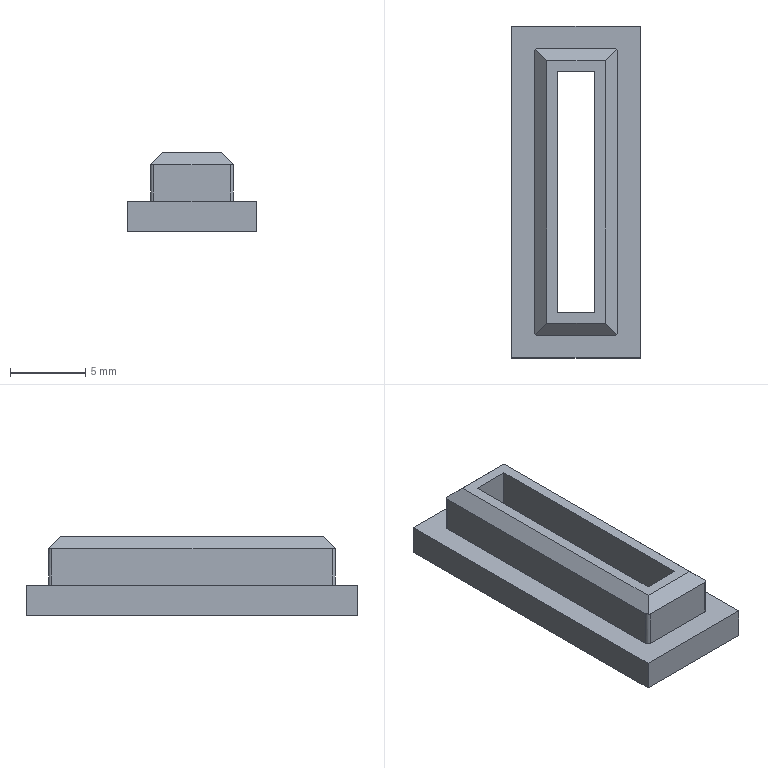Part | NX | features BREP 1 | 1 solid | 23 faces | box 8.5 x 22 x 5.2 mm | volume 485.324 mm3 | plane 19 | cylinder 4 | commonest cylinder face diameters 0.4 x4
STEP:
#1=CARTESIAN_POINT('',(-10.019,-6.965,4.4));
#2=VERTEX_POINT('',#1);
#3=CARTESIAN_POINT('',(-10.077,-7.106,4.459));
#4=VERTEX_POINT('',#3);
#5=CARTESIAN_POINT('',(-10.219,-6.965,4.6));
#6=DIRECTION('',(-0.7071,0.,-0.7071));
#7=DIRECTION('',(0.7071,0.,-0.7071));
#8=AXIS2_PLACEMENT_3D('',#5,#6,#7);
#9=ELLIPSE('',#8,0.2828,0.2);
#10=EDGE_CURVE('',#2,#4,#9,.T.);
#11=ORIENTED_EDGE('',*,*,#10,.F.);
#12=CARTESIAN_POINT('',(-10.019,11.635,4.4));
#13=VERTEX_POINT('',#12);
#14=CARTESIAN_POINT('',(-10.019,11.635,4.4));
#15=DIRECTION('',(0.,-1.,0.));
#16=VECTOR('',#15,1000.);
#17=LINE('',#14,#16);
#18=EDGE_CURVE('',#13,#2,#17,.T.);
#19=ORIENTED_EDGE('',*,*,#18,.F.);
#20=CARTESIAN_POINT('',(-10.078,11.777,4.459));
#21=VERTEX_POINT('',#20);
#22=CARTESIAN_POINT('',(-10.219,11.635,4.6));
#23=DIRECTION('',(-0.7071,0.,-0.7071));
#24=DIRECTION('',(0.7071,0.,-0.7071));
#25=AXIS2_PLACEMENT_3D('',#22,#23,#24);
#26=ELLIPSE('',#25,0.2828,0.2);
#27=EDGE_CURVE('',#21,#13,#26,.T.);
#28=ORIENTED_EDGE('',*,*,#27,.F.);
#29=CARTESIAN_POINT('',(-10.819,11.034,5.2));
#30=VERTEX_POINT('',#29);
#31=CARTESIAN_POINT('',(-10.819,11.034,5.2));
#32=DIRECTION('',(0.5767,0.5786,-0.5767));
#33=VECTOR('',#32,1000.);
#34=LINE('',#31,#33);
#35=EDGE_CURVE('',#30,#21,#34,.T.);
#36=ORIENTED_EDGE('',*,*,#35,.F.);
#37=CARTESIAN_POINT('',(-10.819,-6.367,5.2));
#38=VERTEX_POINT('',#37);
#39=CARTESIAN_POINT('',(-10.819,-6.367,5.2));
#40=DIRECTION('',(0.,1.,0.));
#41=VECTOR('',#40,1000.);
#42=LINE('',#39,#41);
#43=EDGE_CURVE('',#38,#30,#42,.T.);
#44=ORIENTED_EDGE('',*,*,#43,.F.);
#45=CARTESIAN_POINT('',(-10.077,-7.106,4.459));
#46=DIRECTION('',(-0.578,0.5761,0.578));
#47=VECTOR('',#46,1000.);
#48=LINE('',#45,#47);
#49=EDGE_CURVE('',#4,#38,#48,.T.);
#50=ORIENTED_EDGE('',*,*,#49,.F.);
#51=EDGE_LOOP('',(#11,#19,#28,#36,#44,#50));
#52=FACE_BOUND('',#51,.T.);
#53=CARTESIAN_POINT('',(-10.077,-8.665,4.459));
#54=DIRECTION('',(-0.7071,0.,-0.7071));
#55=DIRECTION('',(-0.7071,0.,0.7071));
#56=AXIS2_PLACEMENT_3D('',#53,#54,#55);
#57=PLANE('',#56);
#58=ADVANCED_FACE('',(#52),#57,.F.);
#59=CARTESIAN_POINT('',(-15.519,11.635,4.4));
#60=VERTEX_POINT('',#59);
#61=CARTESIAN_POINT('',(-15.46,11.777,4.459));
#62=VERTEX_POINT('',#61);
#63=CARTESIAN_POINT('',(-15.319,11.635,4.6));
#64=DIRECTION('',(0.7071,0.,-0.7071));
#65=DIRECTION('',(-0.7071,0.,-0.7071));
#66=AXIS2_PLACEMENT_3D('',#63,#64,#65);
#67=ELLIPSE('',#66,0.2828,0.2);
#68=EDGE_CURVE('',#60,#62,#67,.T.);
#69=ORIENTED_EDGE('',*,*,#68,.F.);
#70=CARTESIAN_POINT('',(-15.519,-6.965,4.4));
#71=VERTEX_POINT('',#70);
#72=CARTESIAN_POINT('',(-15.519,-6.965,4.4));
#73=DIRECTION('',(0.,1.,0.));
#74=VECTOR('',#73,1000.);
#75=LINE('',#72,#74);
#76=EDGE_CURVE('',#71,#60,#75,.T.);
#77=ORIENTED_EDGE('',*,*,#76,.F.);
#78=CARTESIAN_POINT('',(-15.46,-7.106,4.459));
#79=VERTEX_POINT('',#78);
#80=CARTESIAN_POINT('',(-15.319,-6.965,4.6));
#81=DIRECTION('',(0.7071,0.,-0.7071));
#82=DIRECTION('',(-0.7071,0.,-0.7071));
#83=AXIS2_PLACEMENT_3D('',#80,#81,#82);
#84=ELLIPSE('',#83,0.2828,0.2);
#85=EDGE_CURVE('',#79,#71,#84,.T.);
#86=ORIENTED_EDGE('',*,*,#85,.F.);
#87=CARTESIAN_POINT('',(-14.719,-6.367,5.2));
#88=VERTEX_POINT('',#87);
#89=CARTESIAN_POINT('',(-14.719,-6.367,5.2));
#90=DIRECTION('',(-0.578,-0.5761,-0.578));
#91=VECTOR('',#90,1000.);
#92=LINE('',#89,#91);
#93=EDGE_CURVE('',#88,#79,#92,.T.);
#94=ORIENTED_EDGE('',*,*,#93,.F.);
#95=CARTESIAN_POINT('',(-14.719,11.034,5.2));
#96=VERTEX_POINT('',#95);
#97=CARTESIAN_POINT('',(-14.719,11.034,5.2));
#98=DIRECTION('',(0.,-1.,0.));
#99=VECTOR('',#98,1000.);
#100=LINE('',#97,#99);
#101=EDGE_CURVE('',#96,#88,#100,.T.);
#102=ORIENTED_EDGE('',*,*,#101,.F.);
#103=CARTESIAN_POINT('',(-15.46,11.777,4.459));
#104=DIRECTION('',(0.5767,-0.5786,0.5767));
#105=VECTOR('',#104,1000.);
#106=LINE('',#103,#105);
#107=EDGE_CURVE('',#62,#96,#106,.T.);
#108=ORIENTED_EDGE('',*,*,#107,.F.);
#109=EDGE_LOOP('',(#69,#77,#86,#94,#102,#108));
#110=FACE_BOUND('',#109,.T.);
#111=CARTESIAN_POINT('',(-15.46,-8.665,4.459));
#112=DIRECTION('',(0.7071,0.,-0.7071));
#113=DIRECTION('',(-0.7071,0.,-0.7071));
#114=AXIS2_PLACEMENT_3D('',#111,#112,#113);
#115=PLANE('',#114);
#116=ADVANCED_FACE('',(#110),#115,.F.);
#117=ORIENTED_EDGE('',*,*,#10,.T.);
#118=CARTESIAN_POINT('',(-10.219,-7.165,4.4));
#119=VERTEX_POINT('',#118);
#120=CARTESIAN_POINT('',(-10.219,-6.965,4.601));
#121=DIRECTION('',(0.,0.7083,-0.7059));
#122=DIRECTION('',(0.,-0.7059,-0.7083));
#123=AXIS2_PLACEMENT_3D('',#120,#121,#122);
#124=ELLIPSE('',#123,0.2833,0.2);
#125=EDGE_CURVE('',#4,#119,#124,.T.);
#126=ORIENTED_EDGE('',*,*,#125,.T.);
#127=CARTESIAN_POINT('',(-10.219,-7.165,2.));
#128=VERTEX_POINT('',#127);
#129=CARTESIAN_POINT('',(-10.219,-7.165,2.));
#130=DIRECTION('',(0.,0.,1.));
#131=VECTOR('',#130,1000.);
#132=LINE('',#129,#131);
#133=EDGE_CURVE('',#128,#119,#132,.T.);
#134=ORIENTED_EDGE('',*,*,#133,.F.);
#135=CARTESIAN_POINT('',(-10.019,-6.965,2.));
#136=VERTEX_POINT('',#135);
#137=CARTESIAN_POINT('',(-10.219,-6.965,2.));
#138=DIRECTION('',(0.,0.,-1.));
#139=DIRECTION('',(0.,-1.,0.));
#140=AXIS2_PLACEMENT_3D('',#137,#138,#139);
#141=CIRCLE('',#140,0.2);
#142=EDGE_CURVE('',#136,#128,#141,.T.);
#143=ORIENTED_EDGE('',*,*,#142,.F.);
#144=CARTESIAN_POINT('',(-10.019,-6.965,2.));
#145=DIRECTION('',(0.,0.,1.));
#146=VECTOR('',#145,1000.);
#147=LINE('',#144,#146);
#148=EDGE_CURVE('',#136,#2,#147,.T.);
#149=ORIENTED_EDGE('',*,*,#148,.T.);
#150=EDGE_LOOP('',(#117,#126,#134,#143,#149));
#151=FACE_BOUND('',#150,.T.);
#152=CARTESIAN_POINT('',(-10.219,-6.965,2.));
#153=DIRECTION('',(0.,0.,1.));
#154=DIRECTION('',(0.,-1.,0.));
#155=AXIS2_PLACEMENT_3D('',#152,#153,#154);
#156=CYLINDRICAL_SURFACE('',#155,0.2);
#157=ADVANCED_FACE('',(#151),#156,.T.);
#158=ORIENTED_EDGE('',*,*,#68,.T.);
#159=CARTESIAN_POINT('',(-15.319,11.835,4.401));
#160=VERTEX_POINT('',#159);
#161=CARTESIAN_POINT('',(-15.319,11.635,4.6));
#162=DIRECTION('',(0.,-0.7059,-0.7083));
#163=DIRECTION('',(0.,0.7083,-0.7059));
#164=AXIS2_PLACEMENT_3D('',#161,#162,#163);
#165=ELLIPSE('',#164,0.2824,0.2);
#166=EDGE_CURVE('',#62,#160,#165,.T.);
#167=ORIENTED_EDGE('',*,*,#166,.T.);
#168=CARTESIAN_POINT('',(-15.319,11.835,2.));
#169=VERTEX_POINT('',#168);
#170=CARTESIAN_POINT('',(-15.319,11.835,2.));
#171=DIRECTION('',(0.,0.,1.));
#172=VECTOR('',#171,1000.);
#173=LINE('',#170,#172);
#174=EDGE_CURVE('',#169,#160,#173,.T.);
#175=ORIENTED_EDGE('',*,*,#174,.F.);
#176=CARTESIAN_POINT('',(-15.519,11.635,2.));
#177=VERTEX_POINT('',#176);
#178=CARTESIAN_POINT('',(-15.319,11.635,2.));
#179=DIRECTION('',(0.,0.,-1.));
#180=DIRECTION('',(0.,1.,0.));
#181=AXIS2_PLACEMENT_3D('',#178,#179,#180);
#182=CIRCLE('',#181,0.2);
#183=EDGE_CURVE('',#177,#169,#182,.T.);
#184=ORIENTED_EDGE('',*,*,#183,.F.);
#185=CARTESIAN_POINT('',(-15.519,11.635,2.));
#186=DIRECTION('',(0.,0.,1.));
#187=VECTOR('',#186,1000.);
#188=LINE('',#185,#187);
#189=EDGE_CURVE('',#177,#60,#188,.T.);
#190=ORIENTED_EDGE('',*,*,#189,.T.);
#191=EDGE_LOOP('',(#158,#167,#175,#184,#190));
#192=FACE_BOUND('',#191,.T.);
#193=CARTESIAN_POINT('',(-15.319,11.635,2.));
#194=DIRECTION('',(0.,0.,1.));
#195=DIRECTION('',(0.,1.,0.));
#196=AXIS2_PLACEMENT_3D('',#193,#194,#195);
#197=CYLINDRICAL_SURFACE('',#196,0.2);
#198=ADVANCED_FACE('',(#192),#197,.T.);
#199=ORIENTED_EDGE('',*,*,#43,.T.);
#200=CARTESIAN_POINT('',(-10.819,11.034,5.2));
#201=DIRECTION('',(-1.,0.,0.));
#202=VECTOR('',#201,1000.);
#203=LINE('',#200,#202);
#204=EDGE_CURVE('',#30,#96,#203,.T.);
#205=ORIENTED_EDGE('',*,*,#204,.T.);
#206=ORIENTED_EDGE('',*,*,#101,.T.);
#207=CARTESIAN_POINT('',(-14.719,-6.367,5.2));
#208=DIRECTION('',(1.,0.,0.));
#209=VECTOR('',#208,1000.);
#210=LINE('',#207,#209);
#211=EDGE_CURVE('',#88,#38,#210,.T.);
#212=ORIENTED_EDGE('',*,*,#211,.T.);
#213=EDGE_LOOP('',(#199,#205,#206,#212));
#214=FACE_BOUND('',#213,.T.);
#215=CARTESIAN_POINT('',(-14.019,-5.665,5.2));
#216=VERTEX_POINT('',#215);
#217=CARTESIAN_POINT('',(-14.019,10.335,5.2));
#218=VERTEX_POINT('',#217);
#219=CARTESIAN_POINT('',(-14.019,-5.665,5.2));
#220=DIRECTION('',(0.,1.,0.));
#221=VECTOR('',#220,1000.);
#222=LINE('',#219,#221);
#223=EDGE_CURVE('',#216,#218,#222,.T.);
#224=ORIENTED_EDGE('',*,*,#223,.T.);
#225=CARTESIAN_POINT('',(-11.519,10.335,5.2));
#226=VERTEX_POINT('',#225);
#227=CARTESIAN_POINT('',(-14.019,10.335,5.2));
#228=DIRECTION('',(1.,0.,0.));
#229=VECTOR('',#228,1000.);
#230=LINE('',#227,#229);
#231=EDGE_CURVE('',#218,#226,#230,.T.);
#232=ORIENTED_EDGE('',*,*,#231,.T.);
#233=CARTESIAN_POINT('',(-11.519,-5.665,5.2));
#234=VERTEX_POINT('',#233);
#235=CARTESIAN_POINT('',(-11.519,10.335,5.2));
#236=DIRECTION('',(0.,-1.,0.));
#237=VECTOR('',#236,1000.);
#238=LINE('',#235,#237);
#239=EDGE_CURVE('',#226,#234,#238,.T.);
#240=ORIENTED_EDGE('',*,*,#239,.T.);
#241=CARTESIAN_POINT('',(-11.519,-5.665,5.2));
#242=DIRECTION('',(-1.,0.,0.));
#243=VECTOR('',#242,1000.);
#244=LINE('',#241,#243);
#245=EDGE_CURVE('',#234,#216,#244,.T.);
#246=ORIENTED_EDGE('',*,*,#245,.T.);
#247=EDGE_LOOP('',(#224,#232,#240,#246));
#248=FACE_BOUND('',#247,.T.);
#249=CARTESIAN_POINT('',(-12.769,-6.812,5.2));
#250=DIRECTION('',(0.,0.,1.));
#251=DIRECTION('',(1.,0.,0.));
#252=AXIS2_PLACEMENT_3D('',#249,#250,#251);
#253=PLANE('',#252);
#254=ADVANCED_FACE('',(#214,#248),#253,.T.);
#255=ORIENTED_EDGE('',*,*,#49,.T.);
#256=ORIENTED_EDGE('',*,*,#211,.F.);
#257=ORIENTED_EDGE('',*,*,#93,.T.);
#258=CARTESIAN_POINT('',(-15.319,-7.165,4.4));
#259=VERTEX_POINT('',#258);
#260=CARTESIAN_POINT('',(-15.319,-6.965,4.601));
#261=DIRECTION('',(0.,0.7083,-0.7059));
#262=DIRECTION('',(0.,-0.7059,-0.7083));
#263=AXIS2_PLACEMENT_3D('',#260,#261,#262);
#264=ELLIPSE('',#263,0.2833,0.2);
#265=EDGE_CURVE('',#259,#79,#264,.T.);
#266=ORIENTED_EDGE('',*,*,#265,.F.);
#267=CARTESIAN_POINT('',(-10.219,-7.165,4.4));
#268=DIRECTION('',(-1.,0.,0.));
#269=VECTOR('',#268,1000.);
#270=LINE('',#267,#269);
#271=EDGE_CURVE('',#119,#259,#270,.T.);
#272=ORIENTED_EDGE('',*,*,#271,.F.);
#273=ORIENTED_EDGE('',*,*,#125,.F.);
#274=EDGE_LOOP('',(#255,#256,#257,#266,#272,#273));
#275=FACE_BOUND('',#274,.T.);
#276=CARTESIAN_POINT('',(-10.019,-7.165,4.4));
#277=DIRECTION('',(0.,0.7083,-0.7059));
#278=DIRECTION('',(-1.,0.,0.));
#279=AXIS2_PLACEMENT_3D('',#276,#277,#278);
#280=PLANE('',#279);
#281=ADVANCED_FACE('',(#275),#280,.F.);
#282=ORIENTED_EDGE('',*,*,#85,.T.);
#283=CARTESIAN_POINT('',(-15.519,-6.965,2.));
#284=VERTEX_POINT('',#283);
#285=CARTESIAN_POINT('',(-15.519,-6.965,2.));
#286=DIRECTION('',(0.,0.,1.));
#287=VECTOR('',#286,1000.);
#288=LINE('',#285,#287);
#289=EDGE_CURVE('',#284,#71,#288,.T.);
#290=ORIENTED_EDGE('',*,*,#289,.F.);
#291=CARTESIAN_POINT('',(-15.319,-7.165,2.));
#292=VERTEX_POINT('',#291);
#293=CARTESIAN_POINT('',(-15.319,-6.965,2.));
#294=DIRECTION('',(0.,0.,-1.));
#295=DIRECTION('',(-1.,-0.000000001,0.));
#296=AXIS2_PLACEMENT_3D('',#293,#294,#295);
#297=CIRCLE('',#296,0.2);
#298=EDGE_CURVE('',#292,#284,#297,.T.);
#299=ORIENTED_EDGE('',*,*,#298,.F.);
#300=CARTESIAN_POINT('',(-15.319,-7.165,2.));
#301=DIRECTION('',(0.,0.,1.));
#302=VECTOR('',#301,1000.);
#303=LINE('',#300,#302);
#304=EDGE_CURVE('',#292,#259,#303,.T.);
#305=ORIENTED_EDGE('',*,*,#304,.T.);
#306=ORIENTED_EDGE('',*,*,#265,.T.);
#307=EDGE_LOOP('',(#282,#290,#299,#305,#306));
#308=FACE_BOUND('',#307,.T.);
#309=CARTESIAN_POINT('',(-15.319,-6.965,2.));
#310=DIRECTION('',(0.,0.,1.));
#311=DIRECTION('',(-1.,-0.000000001,0.));
#312=AXIS2_PLACEMENT_3D('',#309,#310,#311);
#313=CYLINDRICAL_SURFACE('',#312,0.2);
#314=ADVANCED_FACE('',(#308),#313,.T.);
#315=ORIENTED_EDGE('',*,*,#76,.T.);
#316=ORIENTED_EDGE('',*,*,#189,.F.);
#317=CARTESIAN_POINT('',(-15.519,-6.965,2.));
#318=DIRECTION('',(0.,1.,0.));
#319=VECTOR('',#318,1000.);
#320=LINE('',#317,#319);
#321=EDGE_CURVE('',#284,#177,#320,.T.);
#322=ORIENTED_EDGE('',*,*,#321,.F.);
#323=ORIENTED_EDGE('',*,*,#289,.T.);
#324=EDGE_LOOP('',(#315,#316,#322,#323));
#325=FACE_BOUND('',#324,.T.);
#326=CARTESIAN_POINT('',(-15.519,-6.965,2.));
#327=DIRECTION('',(-1.,0.,0.));
#328=DIRECTION('',(0.,0.,1.));
#329=AXIS2_PLACEMENT_3D('',#326,#327,#328);
#330=PLANE('',#329);
#331=ADVANCED_FACE('',(#325),#330,.T.);
#332=ORIENTED_EDGE('',*,*,#35,.T.);
#333=CARTESIAN_POINT('',(-10.219,11.835,4.401));
#334=VERTEX_POINT('',#333);
#335=CARTESIAN_POINT('',(-10.219,11.635,4.6));
#336=DIRECTION('',(0.,-0.7059,-0.7083));
#337=DIRECTION('',(0.,0.7083,-0.7059));
#338=AXIS2_PLACEMENT_3D('',#335,#336,#337);
#339=ELLIPSE('',#338,0.2824,0.2);
#340=EDGE_CURVE('',#334,#21,#339,.T.);
#341=ORIENTED_EDGE('',*,*,#340,.F.);
#342=CARTESIAN_POINT('',(-15.319,11.835,4.401));
#343=DIRECTION('',(1.,0.,0.));
#344=VECTOR('',#343,1000.);
#345=LINE('',#342,#344);
#346=EDGE_CURVE('',#160,#334,#345,.T.);
#347=ORIENTED_EDGE('',*,*,#346,.F.);
#348=ORIENTED_EDGE('',*,*,#166,.F.);
#349=ORIENTED_EDGE('',*,*,#107,.T.);
#350=ORIENTED_EDGE('',*,*,#204,.F.);
#351=EDGE_LOOP('',(#332,#341,#347,#348,#349,#350));
#352=FACE_BOUND('',#351,.T.);
#353=CARTESIAN_POINT('',(-10.019,11.034,5.2));
#354=DIRECTION('',(0.,-0.7059,-0.7083));
#355=DIRECTION('',(-1.,0.,0.));
#356=AXIS2_PLACEMENT_3D('',#353,#354,#355);
#357=PLANE('',#356);
#358=ADVANCED_FACE('',(#352),#357,.F.);
#359=ORIENTED_EDGE('',*,*,#27,.T.);
#360=CARTESIAN_POINT('',(-10.019,11.635,2.));
#361=VERTEX_POINT('',#360);
#362=CARTESIAN_POINT('',(-10.019,11.635,2.));
#363=DIRECTION('',(0.,0.,1.));
#364=VECTOR('',#363,1000.);
#365=LINE('',#362,#364);
#366=EDGE_CURVE('',#361,#13,#365,.T.);
#367=ORIENTED_EDGE('',*,*,#366,.F.);
#368=CARTESIAN_POINT('',(-10.219,11.835,2.));
#369=VERTEX_POINT('',#368);
#370=CARTESIAN_POINT('',(-10.219,11.635,2.));
#371=DIRECTION('',(0.,0.,-1.));
#372=DIRECTION('',(1.,0.,0.));
#373=AXIS2_PLACEMENT_3D('',#370,#371,#372);
#374=CIRCLE('',#373,0.2);
#375=EDGE_CURVE('',#369,#361,#374,.T.);
#376=ORIENTED_EDGE('',*,*,#375,.F.);
#377=CARTESIAN_POINT('',(-10.219,11.835,2.));
#378=DIRECTION('',(0.,0.,1.));
#379=VECTOR('',#378,1000.);
#380=LINE('',#377,#379);
#381=EDGE_CURVE('',#369,#334,#380,.T.);
#382=ORIENTED_EDGE('',*,*,#381,.T.);
#383=ORIENTED_EDGE('',*,*,#340,.T.);
#384=EDGE_LOOP('',(#359,#367,#376,#382,#383));
#385=FACE_BOUND('',#384,.T.);
#386=CARTESIAN_POINT('',(-10.219,11.635,2.));
#387=DIRECTION('',(0.,0.,1.));
#388=DIRECTION('',(1.,0.,0.));
#389=AXIS2_PLACEMENT_3D('',#386,#387,#388);
#390=CYLINDRICAL_SURFACE('',#389,0.2);
#391=ADVANCED_FACE('',(#385),#390,.T.);
#392=ORIENTED_EDGE('',*,*,#18,.T.);
#393=ORIENTED_EDGE('',*,*,#148,.F.);
#394=CARTESIAN_POINT('',(-10.019,11.635,2.));
#395=DIRECTION('',(0.,-1.,0.));
#396=VECTOR('',#395,1000.);
#397=LINE('',#394,#396);
#398=EDGE_CURVE('',#361,#136,#397,.T.);
#399=ORIENTED_EDGE('',*,*,#398,.F.);
#400=ORIENTED_EDGE('',*,*,#366,.T.);
#401=EDGE_LOOP('',(#392,#393,#399,#400));
#402=FACE_BOUND('',#401,.T.);
#403=CARTESIAN_POINT('',(-10.019,11.635,2.));
#404=DIRECTION('',(1.,0.,0.));
#405=DIRECTION('',(0.,0.,-1.));
#406=AXIS2_PLACEMENT_3D('',#403,#404,#405);
#407=PLANE('',#406);
#408=ADVANCED_FACE('',(#402),#407,.T.);
#409=ORIENTED_EDGE('',*,*,#223,.F.);
#410=CARTESIAN_POINT('',(-14.019,-5.665,0.));
#411=VERTEX_POINT('',#410);
#412=CARTESIAN_POINT('',(-14.019,-5.665,5.2));
#413=DIRECTION('',(0.,0.,-1.));
#414=VECTOR('',#413,1000.);
#415=LINE('',#412,#414);
#416=EDGE_CURVE('',#216,#411,#415,.T.);
#417=ORIENTED_EDGE('',*,*,#416,.T.);
#418=CARTESIAN_POINT('',(-14.019,10.335,0.));
#419=VERTEX_POINT('',#418);
#420=CARTESIAN_POINT('',(-14.019,10.335,0.));
#421=DIRECTION('',(0.,-1.,0.));
#422=VECTOR('',#421,1000.);
#423=LINE('',#420,#422);
#424=EDGE_CURVE('',#419,#411,#423,.T.);
#425=ORIENTED_EDGE('',*,*,#424,.F.);
#426=CARTESIAN_POINT('',(-14.019,10.335,0.));
#427=DIRECTION('',(0.,0.,1.));
#428=VECTOR('',#427,1000.);
#429=LINE('',#426,#428);
#430=EDGE_CURVE('',#419,#218,#429,.T.);
#431=ORIENTED_EDGE('',*,*,#430,.T.);
#432=EDGE_LOOP('',(#409,#417,#425,#431));
#433=FACE_BOUND('',#432,.T.);
#434=CARTESIAN_POINT('',(-14.019,-5.665,2.));
#435=DIRECTION('',(-1.,0.,0.));
#436=DIRECTION('',(0.,0.,1.));
#437=AXIS2_PLACEMENT_3D('',#434,#435,#436);
#438=PLANE('',#437);
#439=ADVANCED_FACE('',(#433),#438,.F.);
#440=ORIENTED_EDGE('',*,*,#231,.F.);
#441=ORIENTED_EDGE('',*,*,#430,.F.);
#442=CARTESIAN_POINT('',(-11.519,10.335,0.));
#443=VERTEX_POINT('',#442);
#444=CARTESIAN_POINT('',(-11.519,10.335,0.));
#445=DIRECTION('',(-1.,0.,0.));
#446=VECTOR('',#445,1000.);
#447=LINE('',#444,#446);
#448=EDGE_CURVE('',#443,#419,#447,.T.);
#449=ORIENTED_EDGE('',*,*,#448,.F.);
#450=CARTESIAN_POINT('',(-11.519,10.335,0.));
#451=DIRECTION('',(0.,0.,1.));
#452=VECTOR('',#451,1000.);
#453=LINE('',#450,#452);
#454=EDGE_CURVE('',#443,#226,#453,.T.);
#455=ORIENTED_EDGE('',*,*,#454,.T.);
#456=EDGE_LOOP('',(#440,#441,#449,#455));
#457=FACE_BOUND('',#456,.T.);
#458=CARTESIAN_POINT('',(-14.019,10.335,2.));
#459=DIRECTION('',(0.,1.,0.));
#460=DIRECTION('',(0.,0.,1.));
#461=AXIS2_PLACEMENT_3D('',#458,#459,#460);
#462=PLANE('',#461);
#463=ADVANCED_FACE('',(#457),#462,.F.);
#464=ORIENTED_EDGE('',*,*,#239,.F.);
#465=ORIENTED_EDGE('',*,*,#454,.F.);
#466=CARTESIAN_POINT('',(-11.519,-5.665,0.));
#467=VERTEX_POINT('',#466);
#468=CARTESIAN_POINT('',(-11.519,-5.665,0.));
#469=DIRECTION('',(0.,1.,0.));
#470=VECTOR('',#469,1000.);
#471=LINE('',#468,#470);
#472=EDGE_CURVE('',#467,#443,#471,.T.);
#473=ORIENTED_EDGE('',*,*,#472,.F.);
#474=CARTESIAN_POINT('',(-11.519,-5.665,0.));
#475=DIRECTION('',(0.,0.,1.));
#476=VECTOR('',#475,1000.);
#477=LINE('',#474,#476);
#478=EDGE_CURVE('',#467,#234,#477,.T.);
#479=ORIENTED_EDGE('',*,*,#478,.T.);
#480=EDGE_LOOP('',(#464,#465,#473,#479));
#481=FACE_BOUND('',#480,.T.);
#482=CARTESIAN_POINT('',(-11.519,10.335,2.));
#483=DIRECTION('',(1.,0.,0.));
#484=DIRECTION('',(0.,0.,-1.));
#485=AXIS2_PLACEMENT_3D('',#482,#483,#484);
#486=PLANE('',#485);
#487=ADVANCED_FACE('',(#481),#486,.F.);
#488=ORIENTED_EDGE('',*,*,#245,.F.);
#489=ORIENTED_EDGE('',*,*,#478,.F.);
#490=CARTESIAN_POINT('',(-14.019,-5.665,0.));
#491=DIRECTION('',(1.,0.,0.));
#492=VECTOR('',#491,1000.);
#493=LINE('',#490,#492);
#494=EDGE_CURVE('',#411,#467,#493,.T.);
#495=ORIENTED_EDGE('',*,*,#494,.F.);
#496=ORIENTED_EDGE('',*,*,#416,.F.);
#497=EDGE_LOOP('',(#488,#489,#495,#496));
#498=FACE_BOUND('',#497,.T.);
#499=CARTESIAN_POINT('',(-11.519,-5.665,2.));
#500=DIRECTION('',(0.,-1.,0.));
#501=DIRECTION('',(0.,0.,-1.));
#502=AXIS2_PLACEMENT_3D('',#499,#500,#501);
#503=PLANE('',#502);
#504=ADVANCED_FACE('',(#498),#503,.F.);
#505=ORIENTED_EDGE('',*,*,#346,.T.);
#506=ORIENTED_EDGE('',*,*,#381,.F.);
#507=CARTESIAN_POINT('',(-15.319,11.835,2.));
#508=DIRECTION('',(1.,0.,0.));
#509=VECTOR('',#508,1000.);
#510=LINE('',#507,#509);
#511=EDGE_CURVE('',#169,#369,#510,.T.);
#512=ORIENTED_EDGE('',*,*,#511,.F.);
#513=ORIENTED_EDGE('',*,*,#174,.T.);
#514=EDGE_LOOP('',(#505,#506,#512,#513));
#515=FACE_BOUND('',#514,.T.);
#516=CARTESIAN_POINT('',(-15.319,11.835,2.));
#517=DIRECTION('',(0.,1.,0.));
#518=DIRECTION('',(0.,0.,1.));
#519=AXIS2_PLACEMENT_3D('',#516,#517,#518);
#520=PLANE('',#519);
#521=ADVANCED_FACE('',(#515),#520,.T.);
#522=ORIENTED_EDGE('',*,*,#271,.T.);
#523=ORIENTED_EDGE('',*,*,#304,.F.);
#524=CARTESIAN_POINT('',(-10.219,-7.165,2.));
#525=DIRECTION('',(-1.,0.,0.));
#526=VECTOR('',#525,1000.);
#527=LINE('',#524,#526);
#528=EDGE_CURVE('',#128,#292,#527,.T.);
#529=ORIENTED_EDGE('',*,*,#528,.F.);
#530=ORIENTED_EDGE('',*,*,#133,.T.);
#531=EDGE_LOOP('',(#522,#523,#529,#530));
#532=FACE_BOUND('',#531,.T.);
#533=CARTESIAN_POINT('',(-10.219,-7.165,2.));
#534=DIRECTION('',(0.,-1.,0.));
#535=DIRECTION('',(0.,0.,-1.));
#536=AXIS2_PLACEMENT_3D('',#533,#534,#535);
#537=PLANE('',#536);
#538=ADVANCED_FACE('',(#532),#537,.T.);
#539=CARTESIAN_POINT('',(-17.019,-8.665,2.));
#540=VERTEX_POINT('',#539);
#541=CARTESIAN_POINT('',(-17.019,13.335,2.));
#542=VERTEX_POINT('',#541);
#543=CARTESIAN_POINT('',(-17.019,-8.665,2.));
#544=DIRECTION('',(0.,1.,0.));
#545=VECTOR('',#544,1000.);
#546=LINE('',#543,#545);
#547=EDGE_CURVE('',#540,#542,#546,.T.);
#548=ORIENTED_EDGE('',*,*,#547,.F.);
#549=CARTESIAN_POINT('',(-8.519,-8.665,2.));
#550=VERTEX_POINT('',#549);
#551=CARTESIAN_POINT('',(-8.519,-8.665,2.));
#552=DIRECTION('',(-1.,0.,0.));
#553=VECTOR('',#552,1000.);
#554=LINE('',#551,#553);
#555=EDGE_CURVE('',#550,#540,#554,.T.);
#556=ORIENTED_EDGE('',*,*,#555,.F.);
#557=CARTESIAN_POINT('',(-8.519,13.335,2.));
#558=VERTEX_POINT('',#557);
#559=CARTESIAN_POINT('',(-8.519,13.335,2.));
#560=DIRECTION('',(0.,-1.,0.));
#561=VECTOR('',#560,1000.);
#562=LINE('',#559,#561);
#563=EDGE_CURVE('',#558,#550,#562,.T.);
#564=ORIENTED_EDGE('',*,*,#563,.F.);
#565=CARTESIAN_POINT('',(-17.019,13.335,2.));
#566=DIRECTION('',(1.,0.,0.));
#567=VECTOR('',#566,1000.);
#568=LINE('',#565,#567);
#569=EDGE_CURVE('',#542,#558,#568,.T.);
#570=ORIENTED_EDGE('',*,*,#569,.F.);
#571=EDGE_LOOP('',(#548,#556,#564,#570));
#572=FACE_BOUND('',#571,.T.);
#573=ORIENTED_EDGE('',*,*,#321,.T.);
#574=ORIENTED_EDGE('',*,*,#183,.T.);
#575=ORIENTED_EDGE('',*,*,#511,.T.);
#576=ORIENTED_EDGE('',*,*,#375,.T.);
#577=ORIENTED_EDGE('',*,*,#398,.T.);
#578=ORIENTED_EDGE('',*,*,#142,.T.);
#579=ORIENTED_EDGE('',*,*,#528,.T.);
#580=ORIENTED_EDGE('',*,*,#298,.T.);
#581=EDGE_LOOP('',(#573,#574,#575,#576,#577,#578,#579,#580));
#582=FACE_BOUND('',#581,.T.);
#583=CARTESIAN_POINT('',(-12.769,2.335,2.));
#584=DIRECTION('',(0.,0.,1.));
#585=DIRECTION('',(1.,0.,0.));
#586=AXIS2_PLACEMENT_3D('',#583,#584,#585);
#587=PLANE('',#586);
#588=ADVANCED_FACE('',(#572,#582),#587,.T.);
#589=ORIENTED_EDGE('',*,*,#547,.T.);
#590=CARTESIAN_POINT('',(-17.019,13.335,0.));
#591=VERTEX_POINT('',#590);
#592=CARTESIAN_POINT('',(-17.019,13.335,0.));
#593=DIRECTION('',(0.,0.,1.));
#594=VECTOR('',#593,1000.);
#595=LINE('',#592,#594);
#596=EDGE_CURVE('',#591,#542,#595,.T.);
#597=ORIENTED_EDGE('',*,*,#596,.F.);
#598=CARTESIAN_POINT('',(-17.019,-8.665,0.));
#599=VERTEX_POINT('',#598);
#600=CARTESIAN_POINT('',(-17.019,13.335,0.));
#601=DIRECTION('',(0.,-1.,0.));
#602=VECTOR('',#601,1000.);
#603=LINE('',#600,#602);
#604=EDGE_CURVE('',#591,#599,#603,.T.);
#605=ORIENTED_EDGE('',*,*,#604,.T.);
#606=CARTESIAN_POINT('',(-17.019,-8.665,0.));
#607=DIRECTION('',(0.,0.,1.));
#608=VECTOR('',#607,1000.);
#609=LINE('',#606,#608);
#610=EDGE_CURVE('',#599,#540,#609,.T.);
#611=ORIENTED_EDGE('',*,*,#610,.T.);
#612=EDGE_LOOP('',(#589,#597,#605,#611));
#613=FACE_BOUND('',#612,.T.);
#614=CARTESIAN_POINT('',(-17.019,-8.665,0.));
#615=DIRECTION('',(-1.,0.,0.));
#616=DIRECTION('',(0.,0.,1.));
#617=AXIS2_PLACEMENT_3D('',#614,#615,#616);
#618=PLANE('',#617);
#619=ADVANCED_FACE('',(#613),#618,.T.);
#620=ORIENTED_EDGE('',*,*,#569,.T.);
#621=CARTESIAN_POINT('',(-8.519,13.335,0.));
#622=VERTEX_POINT('',#621);
#623=CARTESIAN_POINT('',(-8.519,13.335,0.));
#624=DIRECTION('',(0.,0.,1.));
#625=VECTOR('',#624,1000.);
#626=LINE('',#623,#625);
#627=EDGE_CURVE('',#622,#558,#626,.T.);
#628=ORIENTED_EDGE('',*,*,#627,.F.);
#629=CARTESIAN_POINT('',(-8.519,13.335,0.));
#630=DIRECTION('',(-1.,0.,0.));
#631=VECTOR('',#630,1000.);
#632=LINE('',#629,#631);
#633=EDGE_CURVE('',#622,#591,#632,.T.);
#634=ORIENTED_EDGE('',*,*,#633,.T.);
#635=ORIENTED_EDGE('',*,*,#596,.T.);
#636=EDGE_LOOP('',(#620,#628,#634,#635));
#637=FACE_BOUND('',#636,.T.);
#638=CARTESIAN_POINT('',(-17.019,13.335,0.));
#639=DIRECTION('',(0.,1.,0.));
#640=DIRECTION('',(0.,0.,1.));
#641=AXIS2_PLACEMENT_3D('',#638,#639,#640);
#642=PLANE('',#641);
#643=ADVANCED_FACE('',(#637),#642,.T.);
#644=ORIENTED_EDGE('',*,*,#563,.T.);
#645=CARTESIAN_POINT('',(-8.519,-8.665,0.));
#646=VERTEX_POINT('',#645);
#647=CARTESIAN_POINT('',(-8.519,-8.665,0.));
#648=DIRECTION('',(0.,0.,1.));
#649=VECTOR('',#648,1000.);
#650=LINE('',#647,#649);
#651=EDGE_CURVE('',#646,#550,#650,.T.);
#652=ORIENTED_EDGE('',*,*,#651,.F.);
#653=CARTESIAN_POINT('',(-8.519,-8.665,0.));
#654=DIRECTION('',(0.,1.,0.));
#655=VECTOR('',#654,1000.);
#656=LINE('',#653,#655);
#657=EDGE_CURVE('',#646,#622,#656,.T.);
#658=ORIENTED_EDGE('',*,*,#657,.T.);
#659=ORIENTED_EDGE('',*,*,#627,.T.);
#660=EDGE_LOOP('',(#644,#652,#658,#659));
#661=FACE_BOUND('',#660,.T.);
#662=CARTESIAN_POINT('',(-8.519,13.335,0.));
#663=DIRECTION('',(1.,0.,0.));
#664=DIRECTION('',(0.,0.,-1.));
#665=AXIS2_PLACEMENT_3D('',#662,#663,#664);
#666=PLANE('',#665);
#667=ADVANCED_FACE('',(#661),#666,.T.);
#668=ORIENTED_EDGE('',*,*,#555,.T.);
#669=ORIENTED_EDGE('',*,*,#610,.F.);
#670=CARTESIAN_POINT('',(-17.019,-8.665,0.));
#671=DIRECTION('',(1.,0.,0.));
#672=VECTOR('',#671,1000.);
#673=LINE('',#670,#672);
#674=EDGE_CURVE('',#599,#646,#673,.T.);
#675=ORIENTED_EDGE('',*,*,#674,.T.);
#676=ORIENTED_EDGE('',*,*,#651,.T.);
#677=EDGE_LOOP('',(#668,#669,#675,#676));
#678=FACE_BOUND('',#677,.T.);
#679=CARTESIAN_POINT('',(-8.519,-8.665,0.));
#680=DIRECTION('',(0.,-1.,0.));
#681=DIRECTION('',(0.,0.,-1.));
#682=AXIS2_PLACEMENT_3D('',#679,#680,#681);
#683=PLANE('',#682);
#684=ADVANCED_FACE('',(#678),#683,.T.);
#685=ORIENTED_EDGE('',*,*,#674,.F.);
#686=ORIENTED_EDGE('',*,*,#604,.F.);
#687=ORIENTED_EDGE('',*,*,#633,.F.);
#688=ORIENTED_EDGE('',*,*,#657,.F.);
#689=EDGE_LOOP('',(#685,#686,#687,#688));
#690=FACE_BOUND('',#689,.T.);
#691=ORIENTED_EDGE('',*,*,#494,.T.);
#692=ORIENTED_EDGE('',*,*,#472,.T.);
#693=ORIENTED_EDGE('',*,*,#448,.T.);
#694=ORIENTED_EDGE('',*,*,#424,.T.);
#695=EDGE_LOOP('',(#691,#692,#693,#694));
#696=FACE_BOUND('',#695,.T.);
#697=CARTESIAN_POINT('',(-12.769,2.335,0.));
#698=DIRECTION('',(0.,0.,1.));
#699=DIRECTION('',(1.,0.,0.));
#700=AXIS2_PLACEMENT_3D('',#697,#698,#699);
#701=PLANE('',#700);
#702=ADVANCED_FACE('',(#690,#696),#701,.F.);
#703=CLOSED_SHELL('',(#58,#116,#157,#198,#254,#281,#314,#331,#358,#391,#408,#439,#463,#487,#504,#521,#538,#588,#619,#643,#667,#684,#702));
#704=MANIFOLD_SOLID_BREP('',#703);
#705=(LENGTH_UNIT()NAMED_UNIT(*)SI_UNIT(.MILLI.,.METRE.));
#706=UNCERTAINTY_MEASURE_WITH_UNIT(LENGTH_MEASURE(0.00001),#705,'','');
#707=(NAMED_UNIT(*)PLANE_ANGLE_UNIT()SI_UNIT($,.RADIAN.));
#708=(NAMED_UNIT(*)SI_UNIT($,.STERADIAN.)SOLID_ANGLE_UNIT());
#709=(GEOMETRIC_REPRESENTATION_CONTEXT(3)GLOBAL_UNCERTAINTY_ASSIGNED_CONTEXT((#706))GLOBAL_UNIT_ASSIGNED_CONTEXT((#705,#707,#708))REPRESENTATION_CONTEXT('',''));
#710=ADVANCED_BREP_SHAPE_REPRESENTATION('',(#704),#709);